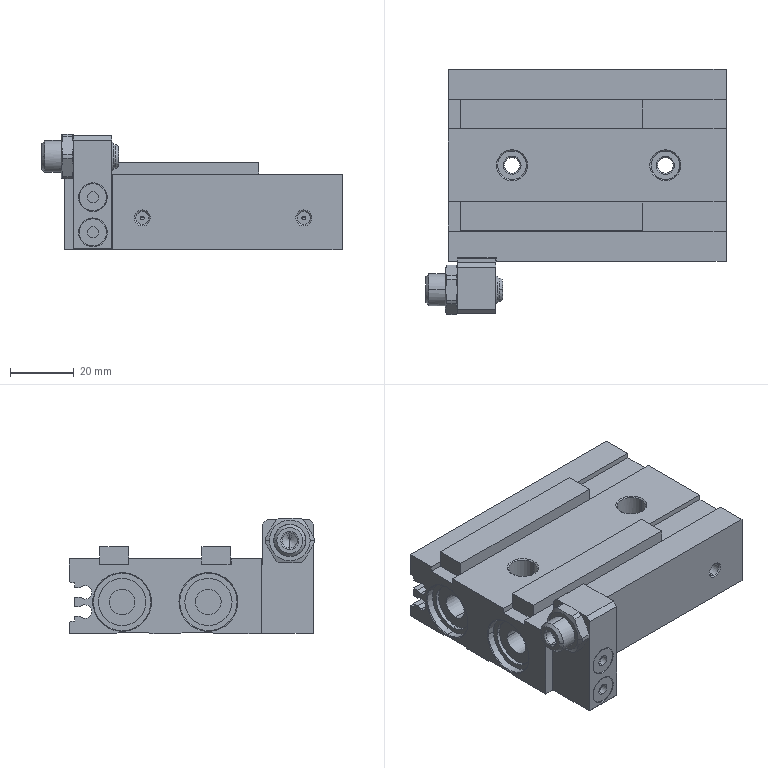Part | SolidWorks | features BaseBody 1 | 1 solid | 253 faces | box 93.95 x 76.75 x 36.25 mm | volume 97741 mm3 | plane 104 | cylinder 91 | cone 54 | spline 4 | commonest cylinder face diameters 4.134 x16 9 x8 4.2 x6 15.5 x6 5 x5 1.2 x4